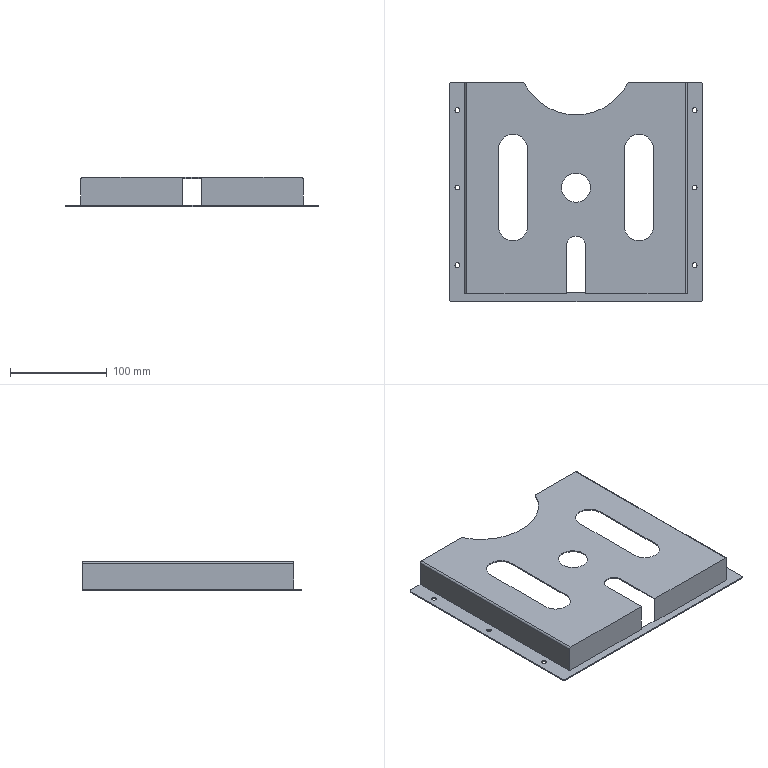Part | SolidWorks | features ICE 4, Fillet 2, Extrusion 1, HoleWzd 1, SketchPattern 1 | 1 solid | 50 faces | box 261 x 226 x 30 mm | volume 80128 mm3 | cylinder 28 | plane 22 | commonest cylinder face diameters 4.8 x12 4 x8 30 x6 20 x1 120 x1